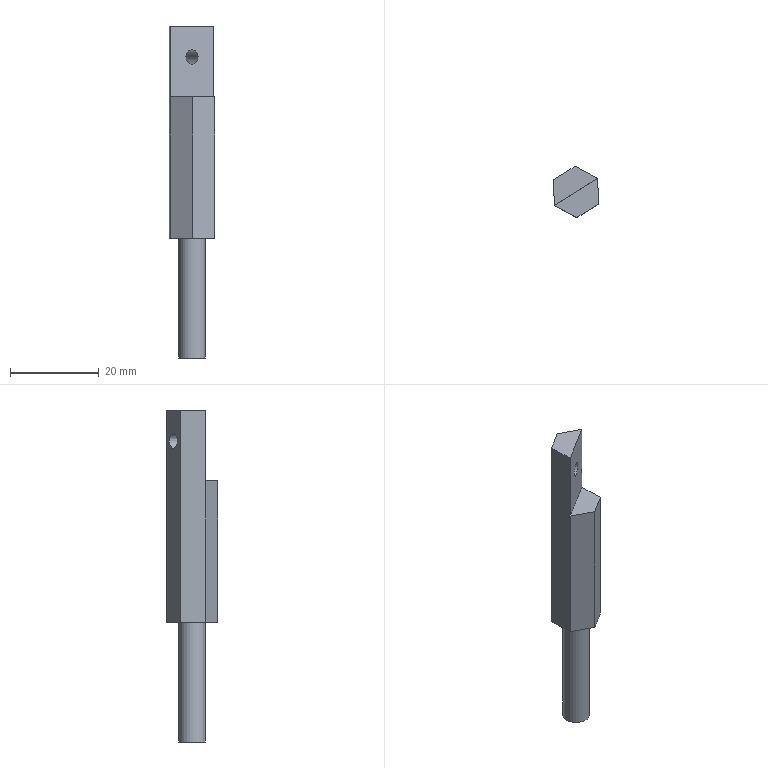Part | NX | features 5003_215_Bracket 2 | 1 solid | 13 faces | box 10.19 x 11.533 x 75 mm | volume 4180 mm3 | plane 11 | cylinder 2 | commonest cylinder face diameters 3.3 x1 6 x1
STEP:
#1=CARTESIAN_POINT('',(218.715,-569.04,-21.5));
#2=VERTEX_POINT('',#1);
#3=CARTESIAN_POINT('',(208.932,-575.155,-21.5));
#4=VERTEX_POINT('',#3);
#5=CARTESIAN_POINT('',(213.823,-572.097,-21.5));
#6=DIRECTION('',(-0.848,-0.5301,0.));
#7=VECTOR('',#6,1000.);
#8=LINE('',#5,#7);
#9=EDGE_CURVE('',#2,#4,#8,.T.);
#10=ORIENTED_EDGE('',*,*,#9,.F.);
#11=CARTESIAN_POINT('',(213.623,-566.334,-21.5));
#12=VERTEX_POINT('',#11);
#13=CARTESIAN_POINT('',(213.623,-566.334,-21.5));
#14=DIRECTION('',(0.883,-0.4693,0.));
#15=VECTOR('',#14,1000.);
#16=LINE('',#13,#15);
#17=EDGE_CURVE('',#12,#2,#16,.T.);
#18=ORIENTED_EDGE('',*,*,#17,.F.);
#19=CARTESIAN_POINT('',(208.73,-569.392,-21.5));
#20=VERTEX_POINT('',#19);
#21=CARTESIAN_POINT('',(208.73,-569.392,-21.5));
#22=DIRECTION('',(0.848,0.5301,0.));
#23=VECTOR('',#22,1000.);
#24=LINE('',#21,#23);
#25=EDGE_CURVE('',#20,#12,#24,.T.);
#26=ORIENTED_EDGE('',*,*,#25,.F.);
#27=CARTESIAN_POINT('',(208.932,-575.158,-21.5));
#28=DIRECTION('',(-0.03507,0.9994,0.));
#29=VECTOR('',#28,1000.);
#30=LINE('',#27,#29);
#31=EDGE_CURVE('',#4,#20,#30,.T.);
#32=ORIENTED_EDGE('',*,*,#31,.F.);
#33=EDGE_LOOP('',(#10,#18,#26,#32));
#34=FACE_BOUND('',#33,.T.);
#35=CARTESIAN_POINT('',(213.825,-572.1,-21.5));
#36=DIRECTION('',(0.,0.,-1.));
#37=DIRECTION('',(0.848,0.5301,0.));
#38=AXIS2_PLACEMENT_3D('',#35,#36,#37);
#39=PLANE('',#38);
#40=ADVANCED_FACE('',(#34),#39,.F.);
#41=CARTESIAN_POINT('',(214.027,-577.866,-69.5));
#42=VERTEX_POINT('',#41);
#43=CARTESIAN_POINT('',(208.932,-575.158,-69.5));
#44=VERTEX_POINT('',#43);
#45=CARTESIAN_POINT('',(214.027,-577.866,-69.5));
#46=DIRECTION('',(-0.883,0.4693,0.));
#47=VECTOR('',#46,1000.);
#48=LINE('',#45,#47);
#49=EDGE_CURVE('',#42,#44,#48,.T.);
#50=ORIENTED_EDGE('',*,*,#49,.T.);
#51=CARTESIAN_POINT('',(208.73,-569.392,-69.5));
#52=VERTEX_POINT('',#51);
#53=CARTESIAN_POINT('',(208.932,-575.158,-69.5));
#54=DIRECTION('',(-0.03507,0.9994,0.));
#55=VECTOR('',#54,1000.);
#56=LINE('',#53,#55);
#57=EDGE_CURVE('',#44,#52,#56,.T.);
#58=ORIENTED_EDGE('',*,*,#57,.T.);
#59=CARTESIAN_POINT('',(213.623,-566.334,-69.5));
#60=VERTEX_POINT('',#59);
#61=CARTESIAN_POINT('',(208.73,-569.392,-69.5));
#62=DIRECTION('',(0.848,0.5301,0.));
#63=VECTOR('',#62,1000.);
#64=LINE('',#61,#63);
#65=EDGE_CURVE('',#52,#60,#64,.T.);
#66=ORIENTED_EDGE('',*,*,#65,.T.);
#67=CARTESIAN_POINT('',(218.718,-569.042,-69.5));
#68=VERTEX_POINT('',#67);
#69=CARTESIAN_POINT('',(213.623,-566.334,-69.5));
#70=DIRECTION('',(0.883,-0.4693,0.));
#71=VECTOR('',#70,1000.);
#72=LINE('',#69,#71);
#73=EDGE_CURVE('',#60,#68,#72,.T.);
#74=ORIENTED_EDGE('',*,*,#73,.T.);
#75=CARTESIAN_POINT('',(218.92,-574.808,-69.5));
#76=VERTEX_POINT('',#75);
#77=CARTESIAN_POINT('',(218.718,-569.042,-69.5));
#78=DIRECTION('',(0.03507,-0.9994,0.));
#79=VECTOR('',#78,1000.);
#80=LINE('',#77,#79);
#81=EDGE_CURVE('',#68,#76,#80,.T.);
#82=ORIENTED_EDGE('',*,*,#81,.T.);
#83=CARTESIAN_POINT('',(218.92,-574.808,-69.5));
#84=DIRECTION('',(-0.848,-0.5301,0.));
#85=VECTOR('',#84,1000.);
#86=LINE('',#83,#85);
#87=EDGE_CURVE('',#76,#42,#86,.T.);
#88=ORIENTED_EDGE('',*,*,#87,.T.);
#89=EDGE_LOOP('',(#50,#58,#66,#74,#82,#88));
#90=FACE_BOUND('',#89,.T.);
#91=CARTESIAN_POINT('',(216.369,-570.51,-69.5));
#92=VERTEX_POINT('',#91);
#93=CARTESIAN_POINT('',(213.825,-572.1,-69.5));
#94=DIRECTION('',(0.,0.,-1.));
#95=DIRECTION('',(0.848,0.5301,0.));
#96=AXIS2_PLACEMENT_3D('',#93,#94,#95);
#97=CIRCLE('',#96,3.);
#98=EDGE_CURVE('',#92,#92,#97,.T.);
#99=ORIENTED_EDGE('',*,*,#98,.F.);
#100=EDGE_LOOP('',(#99));
#101=FACE_BOUND('',#100,.T.);
#102=CARTESIAN_POINT('',(213.825,-572.1,-69.5));
#103=DIRECTION('',(0.,0.,-1.));
#104=DIRECTION('',(0.848,0.5301,0.));
#105=AXIS2_PLACEMENT_3D('',#102,#103,#104);
#106=PLANE('',#105);
#107=ADVANCED_FACE('',(#90,#101),#106,.T.);
#108=CARTESIAN_POINT('',(214.027,-577.866,-37.5));
#109=VERTEX_POINT('',#108);
#110=CARTESIAN_POINT('',(214.027,-577.866,-69.5));
#111=DIRECTION('',(0.,0.,1.));
#112=VECTOR('',#111,1000.);
#113=LINE('',#110,#112);
#114=EDGE_CURVE('',#42,#109,#113,.T.);
#115=ORIENTED_EDGE('',*,*,#114,.T.);
#116=CARTESIAN_POINT('',(208.932,-575.158,-37.5));
#117=VERTEX_POINT('',#116);
#118=CARTESIAN_POINT('',(214.027,-577.866,-37.5));
#119=DIRECTION('',(-0.883,0.4693,0.));
#120=VECTOR('',#119,1000.);
#121=LINE('',#118,#120);
#122=EDGE_CURVE('',#109,#117,#121,.T.);
#123=ORIENTED_EDGE('',*,*,#122,.T.);
#124=CARTESIAN_POINT('',(208.932,-575.158,-69.5));
#125=DIRECTION('',(0.,0.,1.));
#126=VECTOR('',#125,1000.);
#127=LINE('',#124,#126);
#128=EDGE_CURVE('',#44,#117,#127,.T.);
#129=ORIENTED_EDGE('',*,*,#128,.F.);
#130=ORIENTED_EDGE('',*,*,#49,.F.);
#131=EDGE_LOOP('',(#115,#123,#129,#130));
#132=FACE_BOUND('',#131,.T.);
#133=CARTESIAN_POINT('',(214.027,-577.866,-69.5));
#134=DIRECTION('',(0.4693,0.883,0.));
#135=DIRECTION('',(0.883,-0.4693,0.));
#136=AXIS2_PLACEMENT_3D('',#133,#134,#135);
#137=PLANE('',#136);
#138=ADVANCED_FACE('',(#132),#137,.F.);
#139=ORIENTED_EDGE('',*,*,#128,.T.);
#140=CARTESIAN_POINT('',(208.932,-575.155,-37.5));
#141=VERTEX_POINT('',#140);
#142=CARTESIAN_POINT('',(208.932,-575.158,-37.5));
#143=DIRECTION('',(-0.03507,0.9994,0.));
#144=VECTOR('',#143,1000.);
#145=LINE('',#142,#144);
#146=EDGE_CURVE('',#117,#141,#145,.T.);
#147=ORIENTED_EDGE('',*,*,#146,.T.);
#148=CARTESIAN_POINT('',(208.932,-575.155,-69.5));
#149=DIRECTION('',(0.,0.,-1.));
#150=VECTOR('',#149,1000.);
#151=LINE('',#148,#150);
#152=EDGE_CURVE('',#4,#141,#151,.T.);
#153=ORIENTED_EDGE('',*,*,#152,.F.);
#154=ORIENTED_EDGE('',*,*,#31,.T.);
#155=CARTESIAN_POINT('',(208.73,-569.392,-69.5));
#156=DIRECTION('',(0.,0.,1.));
#157=VECTOR('',#156,1000.);
#158=LINE('',#155,#157);
#159=EDGE_CURVE('',#52,#20,#158,.T.);
#160=ORIENTED_EDGE('',*,*,#159,.F.);
#161=ORIENTED_EDGE('',*,*,#57,.F.);
#162=EDGE_LOOP('',(#139,#147,#153,#154,#160,#161));
#163=FACE_BOUND('',#162,.T.);
#164=CARTESIAN_POINT('',(208.932,-575.158,-69.5));
#165=DIRECTION('',(0.9994,0.03507,0.));
#166=DIRECTION('',(0.03507,-0.9994,0.));
#167=AXIS2_PLACEMENT_3D('',#164,#165,#166);
#168=PLANE('',#167);
#169=ADVANCED_FACE('',(#163),#168,.F.);
#170=CARTESIAN_POINT('',(209.776,-568.738,-28.5));
#171=VERTEX_POINT('',#170);
#172=CARTESIAN_POINT('',(211.175,-567.864,-28.5));
#173=DIRECTION('',(0.5301,-0.848,0.));
#174=DIRECTION('',(-0.848,-0.5301,0.));
#175=AXIS2_PLACEMENT_3D('',#172,#173,#174);
#176=CIRCLE('',#175,1.65);
#177=EDGE_CURVE('',#171,#171,#176,.T.);
#178=ORIENTED_EDGE('',*,*,#177,.T.);
#179=EDGE_LOOP('',(#178));
#180=FACE_BOUND('',#179,.T.);
#181=ORIENTED_EDGE('',*,*,#25,.T.);
#182=CARTESIAN_POINT('',(213.623,-566.334,-69.5));
#183=DIRECTION('',(0.,0.,1.));
#184=VECTOR('',#183,1000.);
#185=LINE('',#182,#184);
#186=EDGE_CURVE('',#60,#12,#185,.T.);
#187=ORIENTED_EDGE('',*,*,#186,.F.);
#188=ORIENTED_EDGE('',*,*,#65,.F.);
#189=ORIENTED_EDGE('',*,*,#159,.T.);
#190=EDGE_LOOP('',(#181,#187,#188,#189));
#191=FACE_BOUND('',#190,.T.);
#192=CARTESIAN_POINT('',(208.73,-569.392,-69.5));
#193=DIRECTION('',(0.5301,-0.848,0.));
#194=DIRECTION('',(-0.848,-0.5301,0.));
#195=AXIS2_PLACEMENT_3D('',#192,#193,#194);
#196=PLANE('',#195);
#197=ADVANCED_FACE('',(#180,#191),#196,.F.);
#198=CARTESIAN_POINT('',(218.715,-569.04,-37.5));
#199=VERTEX_POINT('',#198);
#200=CARTESIAN_POINT('',(218.715,-569.04,-69.5));
#201=DIRECTION('',(0.,0.,1.));
#202=VECTOR('',#201,1000.);
#203=LINE('',#200,#202);
#204=EDGE_CURVE('',#199,#2,#203,.T.);
#205=ORIENTED_EDGE('',*,*,#204,.F.);
#206=CARTESIAN_POINT('',(218.718,-569.042,-37.5));
#207=VERTEX_POINT('',#206);
#208=CARTESIAN_POINT('',(213.623,-566.334,-37.5));
#209=DIRECTION('',(0.883,-0.4693,0.));
#210=VECTOR('',#209,1000.);
#211=LINE('',#208,#210);
#212=EDGE_CURVE('',#199,#207,#211,.T.);
#213=ORIENTED_EDGE('',*,*,#212,.T.);
#214=CARTESIAN_POINT('',(218.718,-569.042,-69.5));
#215=DIRECTION('',(0.,0.,1.));
#216=VECTOR('',#215,1000.);
#217=LINE('',#214,#216);
#218=EDGE_CURVE('',#68,#207,#217,.T.);
#219=ORIENTED_EDGE('',*,*,#218,.F.);
#220=ORIENTED_EDGE('',*,*,#73,.F.);
#221=ORIENTED_EDGE('',*,*,#186,.T.);
#222=ORIENTED_EDGE('',*,*,#17,.T.);
#223=EDGE_LOOP('',(#205,#213,#219,#220,#221,#222));
#224=FACE_BOUND('',#223,.T.);
#225=CARTESIAN_POINT('',(213.623,-566.334,-69.5));
#226=DIRECTION('',(-0.4693,-0.883,0.));
#227=DIRECTION('',(-0.883,0.4693,0.));
#228=AXIS2_PLACEMENT_3D('',#225,#226,#227);
#229=PLANE('',#228);
#230=ADVANCED_FACE('',(#224),#229,.F.);
#231=ORIENTED_EDGE('',*,*,#218,.T.);
#232=CARTESIAN_POINT('',(218.92,-574.808,-37.5));
#233=VERTEX_POINT('',#232);
#234=CARTESIAN_POINT('',(218.718,-569.042,-37.5));
#235=DIRECTION('',(0.03507,-0.9994,0.));
#236=VECTOR('',#235,1000.);
#237=LINE('',#234,#236);
#238=EDGE_CURVE('',#207,#233,#237,.T.);
#239=ORIENTED_EDGE('',*,*,#238,.T.);
#240=CARTESIAN_POINT('',(218.92,-574.808,-69.5));
#241=DIRECTION('',(0.,0.,1.));
#242=VECTOR('',#241,1000.);
#243=LINE('',#240,#242);
#244=EDGE_CURVE('',#76,#233,#243,.T.);
#245=ORIENTED_EDGE('',*,*,#244,.F.);
#246=ORIENTED_EDGE('',*,*,#81,.F.);
#247=EDGE_LOOP('',(#231,#239,#245,#246));
#248=FACE_BOUND('',#247,.T.);
#249=CARTESIAN_POINT('',(218.718,-569.042,-69.5));
#250=DIRECTION('',(-0.9994,-0.03507,0.));
#251=DIRECTION('',(-0.03507,0.9994,0.));
#252=AXIS2_PLACEMENT_3D('',#249,#250,#251);
#253=PLANE('',#252);
#254=ADVANCED_FACE('',(#248),#253,.F.);
#255=ORIENTED_EDGE('',*,*,#244,.T.);
#256=CARTESIAN_POINT('',(226.065,-570.342,-37.5));
#257=DIRECTION('',(0.848,0.5301,0.));
#258=VECTOR('',#257,1000.);
#259=LINE('',#256,#258);
#260=EDGE_CURVE('',#109,#233,#259,.T.);
#261=ORIENTED_EDGE('',*,*,#260,.F.);
#262=ORIENTED_EDGE('',*,*,#114,.F.);
#263=ORIENTED_EDGE('',*,*,#87,.F.);
#264=EDGE_LOOP('',(#255,#261,#262,#263));
#265=FACE_BOUND('',#264,.T.);
#266=CARTESIAN_POINT('',(218.92,-574.808,-69.5));
#267=DIRECTION('',(-0.5301,0.848,0.));
#268=DIRECTION('',(0.848,0.5301,0.));
#269=AXIS2_PLACEMENT_3D('',#266,#267,#268);
#270=PLANE('',#269);
#271=ADVANCED_FACE('',(#265),#270,.F.);
#272=CARTESIAN_POINT('',(216.369,-570.51,-96.5));
#273=VERTEX_POINT('',#272);
#274=CARTESIAN_POINT('',(213.825,-572.1,-96.5));
#275=DIRECTION('',(0.,0.,-1.));
#276=DIRECTION('',(0.848,0.5301,0.));
#277=AXIS2_PLACEMENT_3D('',#274,#275,#276);
#278=CIRCLE('',#277,3.);
#279=EDGE_CURVE('',#273,#273,#278,.T.);
#280=ORIENTED_EDGE('',*,*,#279,.F.);
#281=EDGE_LOOP('',(#280));
#282=FACE_BOUND('',#281,.T.);
#283=ORIENTED_EDGE('',*,*,#98,.T.);
#284=EDGE_LOOP('',(#283));
#285=FACE_BOUND('',#284,.T.);
#286=CARTESIAN_POINT('',(213.825,-572.1,-96.5));
#287=DIRECTION('',(0.,0.,1.));
#288=DIRECTION('',(-0.848,-0.5301,0.));
#289=AXIS2_PLACEMENT_3D('',#286,#287,#288);
#290=CYLINDRICAL_SURFACE('',#289,3.);
#291=ADVANCED_FACE('',(#282,#285),#290,.T.);
#292=ORIENTED_EDGE('',*,*,#279,.T.);
#293=EDGE_LOOP('',(#292));
#294=FACE_BOUND('',#293,.T.);
#295=CARTESIAN_POINT('',(213.825,-572.1,-96.5));
#296=DIRECTION('',(0.,0.,-1.));
#297=DIRECTION('',(0.848,0.5301,0.));
#298=AXIS2_PLACEMENT_3D('',#295,#296,#297);
#299=PLANE('',#298);
#300=ADVANCED_FACE('',(#294),#299,.T.);
#301=ORIENTED_EDGE('',*,*,#260,.T.);
#302=ORIENTED_EDGE('',*,*,#238,.F.);
#303=ORIENTED_EDGE('',*,*,#212,.F.);
#304=CARTESIAN_POINT('',(223.415,-566.102,-37.5));
#305=DIRECTION('',(0.848,0.5301,0.));
#306=VECTOR('',#305,1000.);
#307=LINE('',#304,#306);
#308=EDGE_CURVE('',#141,#199,#307,.T.);
#309=ORIENTED_EDGE('',*,*,#308,.F.);
#310=ORIENTED_EDGE('',*,*,#146,.F.);
#311=ORIENTED_EDGE('',*,*,#122,.F.);
#312=EDGE_LOOP('',(#301,#302,#303,#309,#310,#311));
#313=FACE_BOUND('',#312,.T.);
#314=CARTESIAN_POINT('',(223.415,-566.102,-37.5));
#315=DIRECTION('',(0.,0.,-1.));
#316=DIRECTION('',(0.848,0.5301,0.));
#317=AXIS2_PLACEMENT_3D('',#314,#315,#316);
#318=PLANE('',#317);
#319=ADVANCED_FACE('',(#313),#318,.F.);
#320=CARTESIAN_POINT('',(212.423,-572.973,-28.5));
#321=VERTEX_POINT('',#320);
#322=CARTESIAN_POINT('',(213.822,-572.098,-28.5));
#323=DIRECTION('',(0.5301,-0.848,0.));
#324=DIRECTION('',(-0.848,-0.5301,0.));
#325=AXIS2_PLACEMENT_3D('',#322,#323,#324);
#326=CIRCLE('',#325,1.65);
#327=EDGE_CURVE('',#321,#321,#326,.T.);
#328=ORIENTED_EDGE('',*,*,#327,.F.);
#329=EDGE_LOOP('',(#328));
#330=FACE_BOUND('',#329,.T.);
#331=ORIENTED_EDGE('',*,*,#152,.T.);
#332=ORIENTED_EDGE('',*,*,#308,.T.);
#333=ORIENTED_EDGE('',*,*,#204,.T.);
#334=ORIENTED_EDGE('',*,*,#9,.T.);
#335=EDGE_LOOP('',(#331,#332,#333,#334));
#336=FACE_BOUND('',#335,.T.);
#337=CARTESIAN_POINT('',(213.823,-572.097,-21.5));
#338=DIRECTION('',(0.5301,-0.848,0.));
#339=DIRECTION('',(-0.848,-0.5301,0.));
#340=AXIS2_PLACEMENT_3D('',#337,#338,#339);
#341=PLANE('',#340);
#342=ADVANCED_FACE('',(#330,#336),#341,.T.);
#343=ORIENTED_EDGE('',*,*,#327,.T.);
#344=EDGE_LOOP('',(#343));
#345=FACE_BOUND('',#344,.T.);
#346=ORIENTED_EDGE('',*,*,#177,.F.);
#347=EDGE_LOOP('',(#346));
#348=FACE_BOUND('',#347,.T.);
#349=CARTESIAN_POINT('',(213.822,-572.098,-28.5));
#350=DIRECTION('',(0.5301,-0.848,0.));
#351=DIRECTION('',(-0.848,-0.5301,0.));
#352=AXIS2_PLACEMENT_3D('',#349,#350,#351);
#353=CYLINDRICAL_SURFACE('',#352,1.65);
#354=ADVANCED_FACE('',(#345,#348),#353,.F.);
#355=CLOSED_SHELL('',(#40,#107,#138,#169,#197,#230,#254,#271,#291,#300,#319,#342,#354));
#356=MANIFOLD_SOLID_BREP('',#355);
#357=(LENGTH_UNIT()NAMED_UNIT(*)SI_UNIT(.MILLI.,.METRE.));
#358=UNCERTAINTY_MEASURE_WITH_UNIT(LENGTH_MEASURE(0.00001),#357,'','');
#359=(NAMED_UNIT(*)PLANE_ANGLE_UNIT()SI_UNIT($,.RADIAN.));
#360=(NAMED_UNIT(*)SI_UNIT($,.STERADIAN.)SOLID_ANGLE_UNIT());
#361=(GEOMETRIC_REPRESENTATION_CONTEXT(3)GLOBAL_UNCERTAINTY_ASSIGNED_CONTEXT((#358))GLOBAL_UNIT_ASSIGNED_CONTEXT((#357,#359,#360))REPRESENTATION_CONTEXT('',''));
#362=ADVANCED_BREP_SHAPE_REPRESENTATION('',(#356),#361);